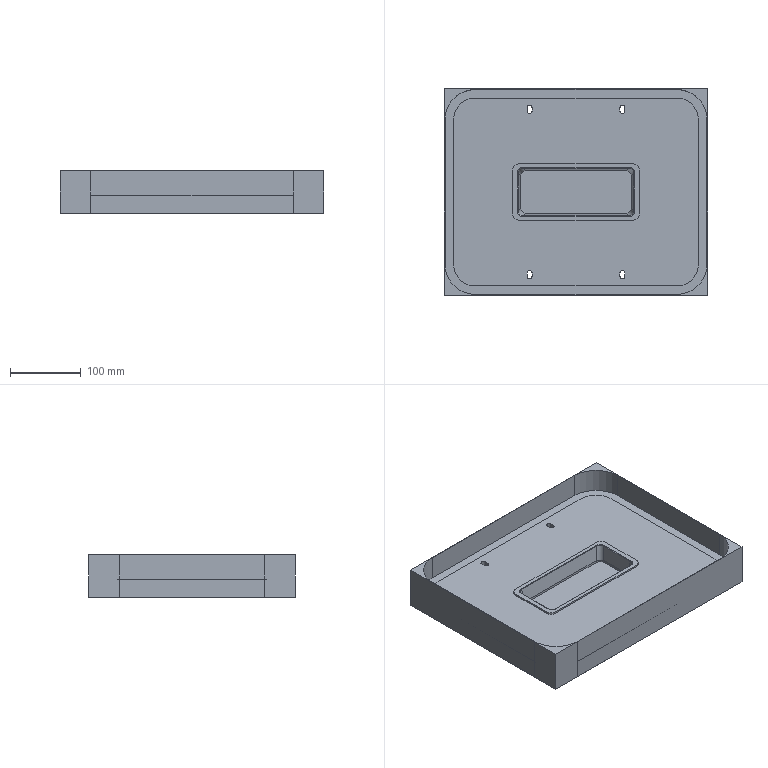NC program | NX | posted with a generic post | part box 371 x 291 x 60.5 mm
Lines 31905 to 32802 of 37416:
(PLANAR_MILL , TOOL : D6)
N63790 M6
N63792 G53
N63794 G17 G0 G90 X-66. Y115.994 S8000 M3 M8
N63796 G43 Z120.5 H0
N63798 Z27.
N63800 G94 G1 Y113.824 Z26.962 F4000.
N63802 X-65.676 Y113.5 Z26.954
N63804 X-65.324 Z26.948
N63806 X-65. Y113.824 Z26.94
N63808 Y119.176 Z26.847
N63810 X-65.324 Y119.5 Z26.839
N63812 X-65.676 Z26.832
N63814 X-66. Y119.176 Z26.824
N63816 Y113.824 Z26.731
N63818 X-65.676 Y113.5 Z26.723
N63820 X-65.324 Z26.717
N63822 X-65. Y113.824 Z26.709
N63824 Y119.176 Z26.615
N63826 X-65.324 Y119.5 Z26.607
N63828 X-65.676 Z26.601
N63830 X-66. Y119.176 Z26.593
N63832 Y113.824 Z26.5
N63834 X-65.676 Y113.5 Z26.492
N63836 X-65.324 Z26.486
N63838 X-65. Y113.824 Z26.478
N63840 Y119.176 Z26.384
N63842 X-65.324 Y119.5 Z26.376
N63844 X-65.676 Z26.37
N63846 X-66. Y119.176 Z26.362
N63848 Y113.824 Z26.269
N63850 X-65.676 Y113.5 Z26.261
N63852 X-65.324 Z26.255
N63854 X-65. Y113.824 Z26.247
N63856 Y119.176 Z26.153
N63858 X-65.324 Y119.5 Z26.145
N63860 X-65.676 Z26.139
N63862 X-66. Y119.176 Z26.131
N63864 Y113.824 Z26.038
N63866 X-65.676 Y113.5 Z26.03
N63868 X-65.324 Z26.024
N63870 X-65. Y113.824 Z26.016
N63872 Y119.176 Z25.922
N63874 X-65.324 Y119.5 Z25.914
N63876 X-65.676 Z25.908
N63878 X-66. Y119.176 Z25.9
N63880 Y113.824 Z25.807
N63882 X-65.676 Y113.5 Z25.799
N63884 X-65.324 Z25.792
N63886 X-65. Y113.824 Z25.784
N63888 Y119.176 Z25.691
N63890 X-65.324 Y119.5 Z25.683
N63892 X-65.676 Z25.677
N63894 X-66. Y119.176 Z25.669
N63896 Y113.824 Z25.575
N63898 X-65.676 Y113.5 Z25.567
N63900 X-65.324 Z25.561
N63902 X-65. Y113.824 Z25.553
N63904 Y119.176 Z25.46
N63906 X-65.324 Y119.5 Z25.452
N63908 X-65.676 Z25.446
N63910 X-66. Y119.176 Z25.438
N63912 Y113.824 Z25.344
N63914 X-65.676 Y113.5 Z25.336
N63916 X-65.324 Z25.33
N63918 X-65. Y113.824 Z25.322
N63920 Y119.176 Z25.229
N63922 X-65.324 Y119.5 Z25.221
N63924 X-65.676 Z25.215
N63926 X-66. Y119.176 Z25.207
N63928 Y113.824 Z25.113
N63930 X-65.676 Y113.5 Z25.105
N63932 X-65.324 Z25.099
N63934 X-65. Y113.824 Z25.091
N63936 Y119.176 Z24.998
N63938 X-65.324 Y119.5 Z24.99
N63940 X-65.676 Z24.984
N63942 X-66. Y119.176 Z24.976
N63944 Y113.824 Z24.882
N63946 X-65.676 Y113.5 Z24.874
N63948 X-65.324 Z24.868
N63950 X-65. Y113.824 Z24.86
N63952 Y119.176 Z24.767
N63954 X-65.324 Y119.5 Z24.759
N63956 X-65.676 Z24.752
N63958 X-66. Y119.176 Z24.744
N63960 Y113.824 Z24.651
N63962 X-65.676 Y113.5 Z24.643
N63964 X-65.324 Z24.637
N63966 X-65. Y113.824 Z24.629
N63968 Y119.176 Z24.535
N63970 X-65.324 Y119.5 Z24.527
N63972 X-65.676 Z24.521
N63974 X-66. Y119.176 Z24.513
N63976 Y113.824 Z24.42
N63978 X-65.676 Y113.5 Z24.412
N63980 X-65.324 Z24.406
N63982 X-65. Y113.824 Z24.398
N63984 Y119.176 Z24.304
N63986 X-65.324 Y119.5 Z24.296
N63988 X-65.676 Z24.29
N63990 X-66. Y119.176 Z24.282
N63992 Y113.824 Z24.189
N63994 X-65.676 Y113.5 Z24.181
N63996 X-65.324 Z24.175
N63998 X-65. Y113.824 Z24.167
N64000 Y119.176 Z24.073
N64002 X-65.324 Y119.5 Z24.065
N64004 X-65.676 Z24.059
N64006 X-66. Y119.176 Z24.051
N64008 Y113.824 Z23.958
N64010 X-65.676 Y113.5 Z23.95
N64012 X-65.324 Z23.944
N64014 X-65. Y113.824 Z23.936
N64016 Y119.176 Z23.842
N64018 X-65.324 Y119.5 Z23.834
N64020 X-65.676 Z23.828
N64022 X-66. Y119.176 Z23.82
N64024 Y113.824 Z23.727
N64026 X-65.676 Y113.5 Z23.719
N64028 X-65.324 Z23.712
N64030 X-65. Y113.824 Z23.704
N64032 Y119.176 Z23.611
N64034 X-65.324 Y119.5 Z23.603
N64036 X-65.676 Z23.597
N64038 X-66. Y119.176 Z23.589
N64040 Y113.824 Z23.495
N64042 X-65.676 Y113.5 Z23.487
N64044 X-65.324 Z23.481
N64046 X-65. Y113.824 Z23.473
N64048 Y119.176 Z23.38
N64050 X-65.324 Y119.5 Z23.372
N64052 X-65.676 Z23.366
N64054 X-66. Y119.176 Z23.358
N64056 Y113.824 Z23.264
N64058 X-65.676 Y113.5 Z23.256
N64060 X-65.324 Z23.25
N64062 X-65. Y113.824 Z23.242
N64064 Y119.176 Z23.149
N64066 X-65.324 Y119.5 Z23.141
N64068 X-65.676 Z23.135
N64070 X-66. Y119.176 Z23.127
N64072 Y113.824 Z23.033
N64074 X-65.676 Y113.5 Z23.025
N64076 X-65.324 Z23.019
N64078 X-65. Y113.824 Z23.011
N64080 Y119.176 Z22.918
N64082 X-65.324 Y119.5 Z22.91
N64084 X-65.676 Z22.904
N64086 X-66. Y119.176 Z22.896
N64088 Y113.824 Z22.802
N64090 X-65.676 Y113.5 Z22.794
N64092 X-65.324 Z22.788
N64094 X-65. Y113.824 Z22.78
N64096 Y119.176 Z22.687
N64098 X-65.324 Y119.5 Z22.679
N64100 X-65.676 Z22.672
N64102 X-66. Y119.176 Z22.664
N64104 Y113.824 Z22.571
N64106 X-65.676 Y113.5 Z22.563
N64108 X-65.324 Z22.557
N64110 X-65. Y113.824 Z22.549
N64112 Y119.176 Z22.455
N64114 X-65.324 Y119.5 Z22.447
N64116 X-65.676 Z22.441
N64118 X-66. Y119.176 Z22.433
N64120 Y113.824 Z22.34
N64122 X-65.676 Y113.5 Z22.332
N64124 X-65.324 Z22.326
N64126 X-65. Y113.824 Z22.318
N64128 Y119.176 Z22.224
N64130 X-65.324 Y119.5 Z22.216
N64132 X-65.676 Z22.21
N64134 X-66. Y119.176 Z22.202
N64136 Y113.824 Z22.109
N64138 X-65.676 Y113.5 Z22.101
N64140 X-65.324 Z22.095
N64142 X-65. Y113.824 Z22.087
N64144 Y119.176 Z21.993
N64146 X-65.324 Y119.5 Z21.985
N64148 X-65.676 Z21.979
N64150 X-66. Y119.176 Z21.971
N64152 Y113.824 Z21.878
N64154 X-65.676 Y113.5 Z21.87
N64156 X-65.324 Z21.864
N64158 X-65. Y113.824 Z21.856
N64160 Y119.176 Z21.762
N64162 X-65.324 Y119.5 Z21.754
N64164 X-65.676 Z21.748
N64166 X-66. Y119.176 Z21.74
N64168 Y113.824 Z21.647
N64170 X-65.676 Y113.5 Z21.639
N64172 X-65.324 Z21.632
N64174 X-65. Y113.824 Z21.624
N64176 Y119.176 Z21.531
N64178 X-65.324 Y119.5 Z21.523
N64180 X-65.676 Z21.517
N64182 X-66. Y119.176 Z21.509
N64184 Y113.824 Z21.415
N64186 X-65.676 Y113.5 Z21.407
N64188 X-65.324 Z21.401
N64190 X-65. Y113.824 Z21.393
N64192 Y119.176 Z21.3
N64194 X-65.324 Y119.5 Z21.292
N64196 X-65.676 Z21.286
N64198 X-66. Y119.176 Z21.278
N64200 Y113.824 Z21.184
N64202 X-65.676 Y113.5 Z21.176
N64204 X-65.324 Z21.17
N64206 X-65. Y113.824 Z21.162
N64208 Y119.176 Z21.069
N64210 X-65.324 Y119.5 Z21.061
N64212 X-65.676 Z21.055
N64214 X-66. Y119.176 Z21.047
N64216 Y113.824 Z20.953
N64218 X-65.676 Y113.5 Z20.945
N64220 X-65.324 Z20.939
N64222 X-65. Y113.824 Z20.931
N64224 Y119.176 Z20.838
N64226 X-65.324 Y119.5 Z20.83
N64228 X-65.676 Z20.824
N64230 X-66. Y119.176 Z20.816
N64232 Y113.824 Z20.722
N64234 X-65.676 Y113.5 Z20.714
N64236 X-65.324 Z20.708
N64238 X-65. Y113.824 Z20.7
N64240 Y119.176 Z20.607
N64242 X-65.324 Y119.5 Z20.599
N64244 X-65.676 Z20.592
N64246 X-66. Y119.176 Z20.584
N64248 Y113.824 Z20.491
N64250 X-65.676 Y113.5 Z20.483
N64252 X-65.324 Z20.477
N64254 X-65. Y113.824 Z20.469
N64256 Y119.176 Z20.375
N64258 X-65.324 Y119.5 Z20.367
N64260 X-65.676 Z20.361
N64262 X-66. Y119.176 Z20.353
N64264 Y113.824 Z20.26
N64266 X-65.676 Y113.5 Z20.252
N64268 X-65.324 Z20.246
N64270 X-65. Y113.824 Z20.238
N64272 Y119.176 Z20.144
N64274 X-65.324 Y119.5 Z20.136
N64276 X-65.676 Z20.13
N64278 X-66. Y119.176 Z20.122
N64280 Y113.824 Z20.029
N64282 X-65.676 Y113.5 Z20.021
N64284 X-65.324 Z20.015
N64286 X-65. Y113.824 Z20.007
N64288 Y119.176 Z19.913
N64290 X-65.324 Y119.5 Z19.905
N64292 X-65.676 Z19.899
N64294 X-66. Y119.176 Z19.891
N64296 Y113.824 Z19.798
N64298 X-65.676 Y113.5 Z19.79
N64300 X-65.324 Z19.784
N64302 X-65. Y113.824 Z19.776
N64304 Y119.176 Z19.682
N64306 X-65.324 Y119.5 Z19.674
N64308 X-65.676 Z19.668
N64310 X-66. Y119.176 Z19.66
N64312 Y113.824 Z19.567
N64314 X-65.676 Y113.5 Z19.559
N64316 X-65.324 Z19.552
N64318 X-65. Y113.824 Z19.544
N64320 Y119.176 Z19.451
N64322 X-65.324 Y119.5 Z19.443
N64324 X-65.676 Z19.437
N64326 X-66. Y119.176 Z19.429
N64328 Y113.824 Z19.335
N64330 X-65.676 Y113.5 Z19.327
N64332 X-65.324 Z19.321
N64334 X-65. Y113.824 Z19.313
N64336 Y119.176 Z19.22
N64338 X-65.324 Y119.5 Z19.212
N64340 X-65.676 Z19.206
N64342 X-66. Y119.176 Z19.198
N64344 Y113.824 Z19.104
N64346 X-65.676 Y113.5 Z19.096
N64348 X-65.324 Z19.09
N64350 X-65. Y113.824 Z19.082
N64352 Y119.176 Z18.989
N64354 X-65.324 Y119.5 Z18.981
N64356 X-65.676 Z18.975
N64358 X-66. Y119.176 Z18.967
N64360 Y113.824 Z18.873
N64362 X-65.676 Y113.5 Z18.865
N64364 X-65.324 Z18.859
N64366 X-65. Y113.824 Z18.851
N64368 Y119.176 Z18.758
N64370 X-65.324 Y119.5 Z18.75
N64372 X-65.676 Z18.744
N64374 X-66. Y119.176 Z18.736
N64376 Y113.824 Z18.642
N64378 X-65.676 Y113.5 Z18.634
N64380 X-65.324 Z18.628
N64382 X-65. Y113.824 Z18.62
N64384 Y119.176 Z18.527
N64386 X-65.324 Y119.5 Z18.519
N64388 X-65.676 Z18.512
N64390 X-66. Y119.176 Z18.504
N64392 Y113.824 Z18.411
N64394 X-65.676 Y113.5 Z18.403
N64396 X-65.324 Z18.397
N64398 X-65. Y113.824 Z18.389
N64400 Y119.176 Z18.295
N64402 X-65.324 Y119.5 Z18.287
N64404 X-65.676 Z18.281
N64406 X-66. Y119.176 Z18.273
N64408 Y113.824 Z18.18
N64410 X-65.676 Y113.5 Z18.172
N64412 X-65.324 Z18.166
N64414 X-65. Y113.824 Z18.158
N64416 Y119.176 Z18.064
N64418 X-65.324 Y119.5 Z18.056
N64420 X-65.676 Z18.05
N64422 X-66. Y119.176 Z18.042
N64424 Y113.824 Z17.949
N64426 X-65.676 Y113.5 Z17.941
N64428 X-65.324 Z17.935
N64430 X-65. Y113.824 Z17.927
N64432 Y119.176 Z17.833
N64434 X-65.324 Y119.5 Z17.825
N64436 X-65.676 Z17.819
N64438 X-66. Y119.176 Z17.811
N64440 Y113.824 Z17.718
N64442 X-65.676 Y113.5 Z17.71
N64444 X-65.324 Z17.704
N64446 X-65. Y113.824 Z17.696
N64448 Y119.176 Z17.602
N64450 X-65.324 Y119.5 Z17.594
N64452 X-65.676 Z17.588
N64454 X-66. Y119.176 Z17.58
N64456 Y113.824 Z17.487
N64458 X-65.676 Y113.5 Z17.479
N64460 X-65.324 Z17.472
N64462 X-65. Y113.824 Z17.464
N64464 Y119.176 Z17.371
N64466 X-65.324 Y119.5 Z17.363
N64468 X-65.676 Z17.357
N64470 X-66. Y119.176 Z17.349
N64472 Y113.824 Z17.255
N64474 X-65.676 Y113.5 Z17.247
N64476 X-65.324 Z17.241
N64478 X-65. Y113.824 Z17.233
N64480 Y119.176 Z17.14
N64482 X-65.324 Y119.5 Z17.132
N64484 X-65.676 Z17.126
N64486 X-66. Y119.176 Z17.118
N64488 Y113.824 Z17.024
N64490 X-65.676 Y113.5 Z17.016
N64492 X-65.324 Z17.01
N64494 X-65. Y113.824 Z17.002
N64496 Y119.176 Z16.909
N64498 X-65.324 Y119.5 Z16.901
N64500 X-65.676 Z16.895
N64502 X-66. Y119.176 Z16.887
N64504 Y113.824 Z16.793
N64506 X-65.676 Y113.5 Z16.785
N64508 X-65.324 Z16.779
N64510 X-65. Y113.824 Z16.771
N64512 Y119.176 Z16.678
N64514 X-65.324 Y119.5 Z16.67
N64516 X-65.676 Z16.664
N64518 X-66. Y119.176 Z16.656
N64520 Y113.824 Z16.562
N64522 X-65.676 Y113.5 Z16.554
N64524 X-65.324 Z16.548
N64526 X-65. Y113.824 Z16.54
N64528 Y119.176 Z16.447
N64530 X-65.324 Y119.5 Z16.439
N64532 X-65.676 Z16.432
N64534 X-66. Y119.176 Z16.424
N64536 Y113.824 Z16.331
N64538 X-65.676 Y113.5 Z16.323
N64540 X-65.324 Z16.317
N64542 X-65. Y113.824 Z16.309
N64544 Y119.176 Z16.215
N64546 X-65.324 Y119.5 Z16.207
N64548 X-65.676 Z16.201
N64550 X-66. Y119.176 Z16.193
N64552 Y113.824 Z16.1
N64554 X-65.676 Y113.5 Z16.092
N64556 X-65.324 Z16.086
N64558 X-65. Y113.824 Z16.078
N64560 Y119.176 Z15.984
N64562 X-65.324 Y119.5 Z15.976
N64564 X-65.676 Z15.97
N64566 X-66. Y119.176 Z15.962
N64568 Y113.824 Z15.869
N64570 X-65.676 Y113.5 Z15.861
N64572 X-65.324 Z15.855
N64574 X-65. Y113.824 Z15.847
N64576 Y119.176 Z15.753
N64578 X-65.324 Y119.5 Z15.745
N64580 X-65.676 Z15.739
N64582 X-66. Y119.176 Z15.731
N64584 Y113.824 Z15.638
N64586 X-65.676 Y113.5 Z15.63
N64588 X-65.324 Z15.624
N64590 X-65. Y113.824 Z15.616
N64592 Y119.176 Z15.522
N64594 X-65.324 Y119.5 Z15.514
N64596 X-65.676 Z15.508
N64598 X-66. Y119.176 Z15.5
N64600 Y113.824 Z15.407
N64602 X-65.676 Y113.5 Z15.399
N64604 X-65.324 Z15.392
N64606 X-65. Y113.824 Z15.384
N64608 Y119.176 Z15.291
N64610 X-65.324 Y119.5 Z15.283
N64612 X-65.676 Z15.277
N64614 X-66. Y119.176 Z15.269
N64616 Y113.824 Z15.175
N64618 X-65.676 Y113.5 Z15.167
N64620 X-65.324 Z15.161
N64622 X-65. Y113.824 Z15.153
N64624 Y119.176 Z15.06
N64626 X-65.324 Y119.5 Z15.052
N64628 X-65.676 Z15.046
N64630 X-66. Y119.176 Z15.038
N64632 Y113.824 Z14.944
N64634 X-65.676 Y113.5 Z14.936
N64636 X-65.324 Z14.93
N64638 X-65. Y113.824 Z14.922
N64640 Y119.176 Z14.829
N64642 X-65.324 Y119.5 Z14.821
N64644 X-65.676 Z14.815
N64646 X-66. Y119.176 Z14.807
N64648 Y113.824 Z14.713
N64650 X-65.676 Y113.5 Z14.705
N64652 X-65.324 Z14.699
N64654 X-65. Y113.824 Z14.691
N64656 Y119.176 Z14.598
N64658 X-65.324 Y119.5 Z14.59
N64660 X-65.676 Z14.584
N64662 X-66. Y119.176 Z14.576
N64664 Y113.824 Z14.482
N64666 X-65.676 Y113.5 Z14.474
N64668 X-65.324 Z14.468
N64670 X-65. Y113.824 Z14.46
N64672 Y119.176 Z14.367
N64674 X-65.324 Y119.5 Z14.359
N64676 X-65.676 Z14.352
N64678 X-66. Y119.176 Z14.344
N64680 Y113.824 Z14.251
N64682 X-65.676 Y113.5 Z14.243
N64684 X-65.324 Z14.237
N64686 X-65. Y113.824 Z14.229
N64688 Y119.176 Z14.135
N64690 X-65.324 Y119.5 Z14.127
N64692 X-65.676 Z14.121
N64694 X-66. Y119.176 Z14.113
N64696 Y113.824 Z14.02
N64698 X-65.676 Y113.5 Z14.012
N64700 X-65.324 Z14.006
N64702 X-65. Y113.824 Z13.998
N64704 Y119.176 Z13.904
N64706 X-65.324 Y119.5 Z13.896
N64708 X-65.676 Z13.89
N64710 X-66. Y119.176 Z13.882
N64712 Y113.824 Z13.789
N64714 X-65.676 Y113.5 Z13.781
N64716 X-65.324 Z13.775
N64718 X-65. Y113.824 Z13.767
N64720 Y119.176 Z13.673
N64722 X-65.324 Y119.5 Z13.665
N64724 X-65.676 Z13.659
N64726 X-66. Y119.176 Z13.651
N64728 Y113.824 Z13.558
N64730 X-65.676 Y113.5 Z13.55
N64732 X-65.324 Z13.544
N64734 X-65. Y113.824 Z13.536
N64736 Y119.176 Z13.442
N64738 X-65.324 Y119.5 Z13.434
N64740 X-65.676 Z13.428
N64742 X-66. Y119.176 Z13.42
N64744 Y113.824 Z13.327
N64746 X-65.676 Y113.5 Z13.319
N64748 X-65.324 Z13.312
N64750 X-65. Y113.824 Z13.304
N64752 Y119.176 Z13.211
N64754 X-65.324 Y119.5 Z13.203
N64756 X-65.676 Z13.197
N64758 X-66. Y119.176 Z13.189
N64760 Y113.824 Z13.095
N64762 X-65.676 Y113.5 Z13.087
N64764 X-65.324 Z13.081
N64766 X-65. Y113.824 Z13.073
N64768 Y119.176 Z12.98
N64770 X-65.324 Y119.5 Z12.972
N64772 X-65.676 Z12.966
N64774 X-66. Y119.176 Z12.958
N64776 Y113.824 Z12.864
N64778 X-65.676 Y113.5 Z12.856
N64780 X-65.324 Z12.85
N64782 X-65. Y113.824 Z12.842
N64784 Y119.176 Z12.749
N64786 X-65.324 Y119.5 Z12.741
N64788 X-65.676 Z12.735
N64790 X-66. Y119.176 Z12.727
N64792 Y113.824 Z12.633
N64794 X-65.676 Y113.5 Z12.625
N64796 X-65.324 Z12.619
N64798 X-65. Y113.824 Z12.611
N64800 Y119.176 Z12.518
N64802 X-65.324 Y119.5 Z12.51
N64804 X-65.676 Z12.504
N64806 X-66. Y119.176 Z12.496
N64808 Y113.824 Z12.402
N64810 X-65.676 Y113.5 Z12.394
N64812 X-65.324 Z12.388
N64814 X-65. Y113.824 Z12.38
N64816 Y119.176 Z12.287
N64818 X-65.324 Y119.5 Z12.279
N64820 X-65.676 Z12.272
N64822 X-66. Y119.176 Z12.264
N64824 Y113.824 Z12.171
N64826 X-65.676 Y113.5 Z12.163
N64828 X-65.324 Z12.157
N64830 X-65. Y113.824 Z12.149
N64832 Y119.176 Z12.055
N64834 X-65.324 Y119.5 Z12.047
N64836 X-65.676 Z12.041
N64838 X-66. Y119.176 Z12.033
N64840 Y113.824 Z11.94
N64842 X-65.676 Y113.5 Z11.932
N64844 X-65.324 Z11.926
N64846 X-65. Y113.824 Z11.918
N64848 Y119.176 Z11.824
N64850 X-65.324 Y119.5 Z11.816
N64852 X-65.676 Z11.81
N64854 X-66. Y119.176 Z11.802
N64856 Y113.824 Z11.709
N64858 X-65.676 Y113.5 Z11.701
N64860 X-65.324 Z11.695
N64862 X-65. Y113.824 Z11.687
N64864 Y119.176 Z11.593
N64866 X-65.324 Y119.5 Z11.585
N64868 X-65.676 Z11.579
N64870 X-66. Y119.176 Z11.571
N64872 Y113.824 Z11.478
N64874 X-65.676 Y113.5 Z11.47
N64876 X-65.324 Z11.464
N64878 X-65. Y113.824 Z11.456
N64880 Y119.176 Z11.362
N64882 X-65.324 Y119.5 Z11.354
N64884 X-65.676 Z11.348
N64886 X-66. Y119.176 Z11.34
N64888 Y113.824 Z11.247
N64890 X-65.676 Y113.5 Z11.239
N64892 X-65.324 Z11.232
N64894 X-65. Y113.824 Z11.224
N64896 Y119.176 Z11.131
N64898 X-65.324 Y119.5 Z11.123
N64900 X-65.676 Z11.117
N64902 X-66. Y119.176 Z11.109
N64904 Y113.824 Z11.015
N64906 X-65.676 Y113.5 Z11.007
N64908 X-65.324 Z11.001
N64910 X-65. Y113.824 Z10.993
N64912 Y119.176 Z10.9
N64914 X-65.324 Y119.5 Z10.892
N64916 X-65.676 Z10.886
N64918 X-66. Y119.176 Z10.878
N64920 Y113.824 Z10.784
N64922 X-65.676 Y113.5 Z10.776
N64924 X-65.324 Z10.77
N64926 X-65. Y113.824 Z10.762
N64928 Y119.176 Z10.669
N64930 X-65.324 Y119.5 Z10.661
N64932 X-65.676 Z10.655
N64934 X-66. Y119.176 Z10.647
N64936 Y113.824 Z10.553
N64938 X-65.676 Y113.5 Z10.545
N64940 X-65.324 Z10.539
N64942 X-65. Y113.824 Z10.531
N64944 Y119.176 Z10.438
N64946 X-65.324 Y119.5 Z10.43
N64948 X-65.676 Z10.424
N64950 X-66. Y119.176 Z10.416
N64952 Y113.824 Z10.322
N64954 X-65.676 Y113.5 Z10.314
N64956 X-65.324 Z10.308
N64958 X-65. Y113.824 Z10.3
N64960 Y119.176 Z10.207
N64962 X-65.324 Y119.5 Z10.199
N64964 X-65.676 Z10.192
N64966 X-66. Y119.176 Z10.184
N64968 Y113.824 Z10.091
N64970 X-65.676 Y113.5 Z10.083
N64972 X-65.324 Z10.077
N64974 X-65. Y113.824 Z10.069
N64976 Y119.176 Z9.975
N64978 X-65.324 Y119.5 Z9.967
N64980 X-65.676 Z9.961
N64982 X-66. Y119.176 Z9.953
N64984 Y113.824 Z9.86
N64986 X-65.676 Y113.5 Z9.852
N64988 X-65.324 Z9.846
N64990 X-65. Y113.824 Z9.838
N64992 Y119.176 Z9.744
N64994 X-65.324 Y119.5 Z9.736
N64996 X-65.676 Z9.73
N64998 X-66. Y119.176 Z9.722
N65000 Y113.824 Z9.629
N65002 X-65.676 Y113.5 Z9.621
N65004 X-65.324 Z9.615
N65006 X-65. Y113.824 Z9.607
N65008 Y119.176 Z9.513
N65010 X-65.324 Y119.5 Z9.505
N65012 X-65.676 Z9.499
N65014 X-66. Y119.176 Z9.491
N65016 Y113.824 Z9.398
N65018 X-65.676 Y113.5 Z9.39
N65020 X-65.324 Z9.384
N65022 X-65. Y113.824 Z9.376
N65024 Y119.176 Z9.282
N65026 X-65.324 Y119.5 Z9.274
N65028 X-65.676 Z9.268
N65030 X-66. Y119.176 Z9.26
N65032 Y113.824 Z9.167
N65034 X-65.676 Y113.5 Z9.159
N65036 X-65.324 Z9.152
N65038 X-65. Y113.824 Z9.144
N65040 Y119.176 Z9.051
N65042 X-65.324 Y119.5 Z9.043
N65044 X-65.676 Z9.037
N65046 X-66. Y119.176 Z9.029
N65048 Y113.824 Z8.935
N65050 X-65.676 Y113.5 Z8.927
N65052 X-65.324 Z8.921
N65054 X-65. Y113.824 Z8.913
N65056 Y119.176 Z8.82
N65058 X-65.324 Y119.5 Z8.812
N65060 X-65.676 Z8.806
N65062 X-66. Y119.176 Z8.798
N65064 Y113.824 Z8.704
N65066 X-65.676 Y113.5 Z8.696
N65068 X-65.324 Z8.69
N65070 X-65. Y113.824 Z8.682
N65072 Y119.176 Z8.589
N65074 X-65.324 Y119.5 Z8.581
N65076 X-65.676 Z8.575
N65078 X-66. Y119.176 Z8.567
N65080 Y113.824 Z8.473
N65082 X-65.676 Y113.5 Z8.465
N65084 X-65.324 Z8.459
N65086 X-65. Y113.824 Z8.451
N65088 Y119.176 Z8.358
N65090 X-65.324 Y119.5 Z8.35
N65092 X-65.676 Z8.344
N65094 X-66. Y119.176 Z8.336
N65096 Y113.824 Z8.242
N65098 X-65.676 Y113.5 Z8.234
N65100 X-65.324 Z8.228
N65102 X-65. Y113.824 Z8.22
N65104 Y119.176 Z8.127
N65106 X-65.324 Y119.5 Z8.119
N65108 X-65.676 Z8.112
N65110 X-66. Y119.176 Z8.104
N65112 Y113.824 Z8.011
N65114 X-65.676 Y113.5 Z8.003
N65116 X-65.324 Z7.997
N65118 X-65. Y113.824 Z7.989
N65120 Y119.176 Z7.895
N65122 X-65.324 Y119.5 Z7.887
N65124 X-65.676 Z7.881
N65126 X-66. Y119.176 Z7.873
N65128 Y113.824 Z7.78
N65130 X-65.676 Y113.5 Z7.772
N65132 X-65.324 Z7.766
N65134 X-65. Y113.824 Z7.758
N65136 Y119.176 Z7.664
N65138 X-65.324 Y119.5 Z7.656
N65140 X-65.676 Z7.65
N65142 X-66. Y119.176 Z7.642
N65144 Y113.824 Z7.549
N65146 X-65.676 Y113.5 Z7.541
N65148 X-65.324 Z7.535
N65150 X-65. Y113.824 Z7.527
N65152 Y119.176 Z7.433
N65154 X-65.324 Y119.5 Z7.425
N65156 X-65.676 Z7.419
N65158 X-66. Y119.176 Z7.411
N65160 Y113.824 Z7.318
N65162 X-65.676 Y113.5 Z7.31
N65164 X-65.324 Z7.304
N65166 X-65. Y113.824 Z7.296
N65168 Y119.176 Z7.202
N65170 X-65.324 Y119.5 Z7.194
N65172 X-65.676 Z7.188
N65174 X-66. Y119.176 Z7.18
N65176 Y113.824 Z7.087
N65178 X-65.676 Y113.5 Z7.079
N65180 X-65.324 Z7.072
N65182 X-65. Y113.824 Z7.064
N65184 Y119.176 Z6.971
N65186 X-65.324 Y119.5 Z6.963
N65188 X-65.676 Z6.957
N65190 X-66. Y119.176 Z6.949
N65192 Y113.824 Z6.856
N65194 X-65.676 Y113.5 Z6.847
N65196 X-65.324 Z6.841
N65198 X-65. Y113.824 Z6.833
N65200 Y119.176 Z6.74
N65202 X-65.324 Y119.5 Z6.732
N65204 X-65.676 Z6.726
N65206 X-66. Y119.176 Z6.718
N65208 Y113.824 Z6.624
N65210 X-65.676 Y113.5 Z6.616
N65212 X-65.324 Z6.61
N65214 X-65. Y113.824 Z6.602
N65216 Y119.176 Z6.509
N65218 X-65.324 Y119.5 Z6.501
N65220 X-65.676 Z6.495
N65222 X-66. Y119.176 Z6.487
N65224 Y113.824 Z6.393
N65226 X-65.676 Y113.5 Z6.385
N65228 X-65.324 Z6.379
N65230 X-65. Y113.824 Z6.371
N65232 Y119.176 Z6.278
N65234 X-65.324 Y119.5 Z6.27
N65236 X-65.676 Z6.264
N65238 X-66. Y119.176 Z6.256
N65240 Y113.824 Z6.162
N65242 X-65.676 Y113.5 Z6.154
N65244 X-65.324 Z6.148
N65246 X-65. Y113.824 Z6.14
N65248 Y119.176 Z6.047
N65250 X-65.324 Y119.5 Z6.039
N65252 X-65.676 Z6.032
N65254 X-66. Y119.176 Z6.024
N65256 Y113.824 Z5.931
N65258 X-65.676 Y113.5 Z5.923
N65260 X-65.324 Z5.917
N65262 X-65. Y113.824 Z5.909
N65264 Y119.176 Z5.816
N65266 X-65.324 Y119.5 Z5.808
N65268 X-65.676 Z5.801
N65270 X-66. Y119.176 Z5.793
N65272 Y113.824 Z5.7
N65274 X-65.676 Y113.5 Z5.692
N65276 X-65.324 Z5.686
N65278 X-65. Y113.824 Z5.678
N65280 Y119.176 Z5.584
N65282 X-65.324 Y119.5 Z5.576
N65284 X-65.676 Z5.57
N65286 X-66. Y119.176 Z5.562
N65288 Y113.824 Z5.469
N65290 X-65.676 Y113.5 Z5.461
N65292 X-65.324 Z5.455
N65294 X-65. Y113.824 Z5.447
N65296 Y119.176 Z5.353
N65298 X-65.324 Y119.5 Z5.345
N65300 X-65.676 Z5.339
N65302 X-66. Y119.176 Z5.331
N65304 Y113.824 Z5.238
N65306 X-65.676 Y113.5 Z5.23
N65308 X-65.324 Z5.224
N65310 X-65. Y113.824 Z5.216
N65312 Y119.176 Z5.122
N65314 X-65.324 Y119.5 Z5.114
N65316 X-65.676 Z5.108
N65318 X-66. Y119.176 Z5.1
N65320 Y113.824 Z5.007
N65322 X-65.676 Y113.5 Z4.999
N65324 X-65.324 Z4.992
N65326 X-65. Y113.824 Z4.984
N65328 Y119.176 Z4.891
N65330 X-65.324 Y119.5 Z4.883
N65332 X-65.676 Z4.877
N65334 X-66. Y119.176 Z4.869
N65336 Y113.824 Z4.776
N65338 X-65.676 Y113.5 Z4.768
N65340 X-65.324 Z4.761
N65342 X-65. Y113.824 Z4.753
N65344 Y119.176 Z4.66
N65346 X-65.324 Y119.5 Z4.652
N65348 X-65.676 Z4.646
N65350 X-66. Y119.176 Z4.638
N65352 Y113.824 Z4.544
N65354 X-65.676 Y113.5 Z4.536
N65356 X-65.324 Z4.53
N65358 X-65. Y113.824 Z4.522
N65360 Y119.176 Z4.429
N65362 X-65.324 Y119.5 Z4.421
N65364 X-65.676 Z4.415
N65366 X-66. Y119.176 Z4.407
N65368 Y113.824 Z4.313
N65370 X-65.676 Y113.5 Z4.305
N65372 X-65.324 Z4.299
N65374 X-65. Y113.824 Z4.291
N65376 Y119.176 Z4.198
N65378 X-65.324 Y119.5 Z4.19
N65380 X-65.676 Z4.184
N65382 X-66. Y119.176 Z4.176
N65384 Y113.824 Z4.082
N65386 X-65.676 Y113.5 Z4.074
N65388 X-65.324 Z4.068
N65390 X-65. Y113.824 Z4.06
N65392 Y119.176 Z3.967
N65394 X-65.324 Y119.5 Z3.959
N65396 X-65.676 Z3.952
N65398 X-66. Y119.176 Z3.944
N65400 Y113.824 Z3.851
N65402 X-65.676 Y113.5 Z3.843
N65404 X-65.324 Z3.837
N65406 X-65. Y113.824 Z3.829
N65408 Y119.176 Z3.736
N65410 X-65.324 Y119.5 Z3.728
N65412 X-65.676 Z3.721
N65414 X-66. Y119.176 Z3.713
N65416 Y113.824 Z3.62
N65418 X-65.676 Y113.5 Z3.612
N65420 X-65.324 Z3.606
N65422 X-65. Y113.824 Z3.598
N65424 Y119.176 Z3.504
N65426 X-65.324 Y119.5 Z3.496
N65428 X-65.676 Z3.49
N65430 X-66. Y119.176 Z3.482
N65432 Y113.824 Z3.389
N65434 X-65.676 Y113.5 Z3.381
N65436 X-65.324 Z3.375
N65438 X-65. Y113.824 Z3.367
N65440 Y119.176 Z3.273
N65442 X-65.324 Y119.5 Z3.265
N65444 X-65.676 Z3.259
N65446 X-66. Y119.176 Z3.251
N65448 Y113.824 Z3.158
N65450 X-65.676 Y113.5 Z3.15
N65452 X-65.324 Z3.144
N65454 X-65. Y113.824 Z3.136
N65456 Y119.176 Z3.042
N65458 X-65.324 Y119.5 Z3.034
N65460 X-65.676 Z3.028
N65462 X-66. Y119.176 Z3.02
N65464 Y113.824 Z2.927
N65466 X-65.676 Y113.5 Z2.919
N65468 X-65.324 Z2.912
N65470 X-65. Y113.824 Z2.904
N65472 Y119.176 Z2.811
N65474 X-65.324 Y119.5 Z2.803
N65476 X-65.676 Z2.797
N65478 X-66. Y119.176 Z2.789
N65480 Y113.824 Z2.696
N65482 X-65.676 Y113.5 Z2.688
N65484 X-65.324 Z2.681
N65486 X-65. Y113.824 Z2.673
N65488 Y119.176 Z2.58
N65490 X-65.324 Y119.5 Z2.572
N65492 X-65.676 Z2.566
N65494 X-66. Y119.176 Z2.558
N65496 Y113.824 Z2.464
N65498 X-65.676 Y113.5 Z2.456
N65500 X-65.324 Z2.45
N65502 X-65. Y113.824 Z2.442
N65504 Y119.176 Z2.349
N65506 X-65.324 Y119.5 Z2.341
N65508 X-65.676 Z2.335
N65510 X-66. Y119.176 Z2.327
N65512 Y113.824 Z2.233
N65514 X-65.676 Y113.5 Z2.225
N65516 X-65.324 Z2.219
N65518 X-65. Y113.824 Z2.211
N65520 Y119.176 Z2.118
N65522 X-65.324 Y119.5 Z2.11
N65524 X-65.676 Z2.104
N65526 X-66. Y119.176 Z2.096
N65528 Y113.824 Z2.002
N65530 X-65.676 Y113.5 Z1.994
N65532 X-65.324 Z1.988
N65534 X-65. Y113.824 Z1.98
N65536 Y119.176 Z1.887
N65538 X-65.324 Y119.5 Z1.879
N65540 X-65.676 Z1.872
N65542 X-66. Y119.176 Z1.864
N65544 Y113.824 Z1.771
N65546 X-65.676 Y113.5 Z1.763
N65548 X-65.324 Z1.757
N65550 X-65. Y113.824 Z1.749
N65552 Y119.176 Z1.656
N65554 X-65.324 Y119.5 Z1.648
N65556 X-65.676 Z1.641
N65558 X-66. Y119.176 Z1.633
N65560 Y113.824 Z1.54
N65562 X-65.676 Y113.5 Z1.532
N65564 X-65.324 Z1.526
N65566 X-65. Y113.824 Z1.518
N65568 Y119.176 Z1.424
N65570 X-65.324 Y119.5 Z1.416
N65572 X-65.676 Z1.41
N65574 X-66. Y119.176 Z1.402
N65576 Y113.824 Z1.309
N65578 X-65.676 Y113.5 Z1.301